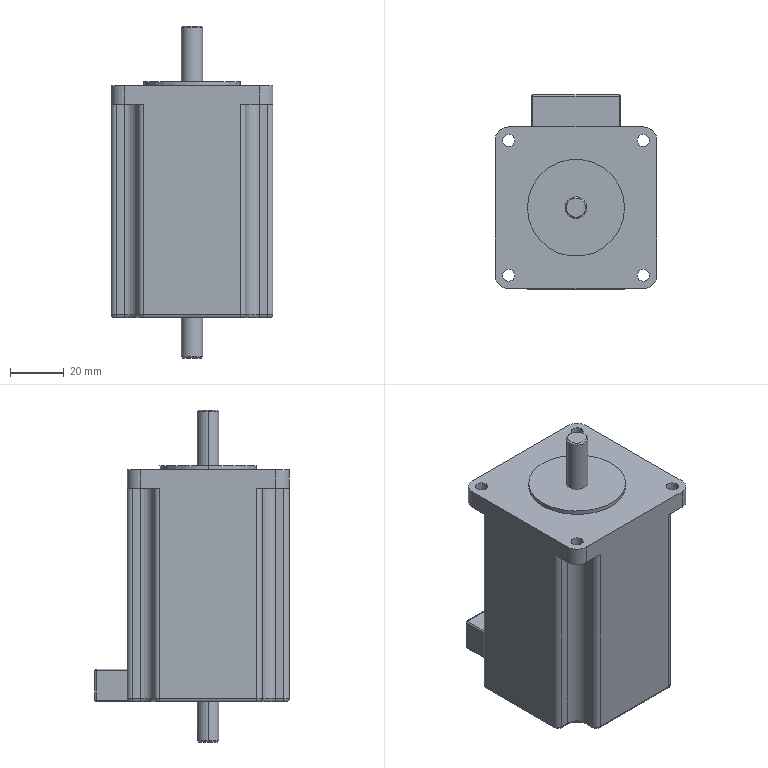Part | NX | 1 solid | 98 faces | box 60 x 72 x 123.1 mm | volume 286563 mm3 | cylinder 51 | plane 27 | torus 12 | sphere 4 | cone 4 | commonest cylinder face diameters 2 x12 1 x9 4 x8 4.5 x8 10 x8 8 x4